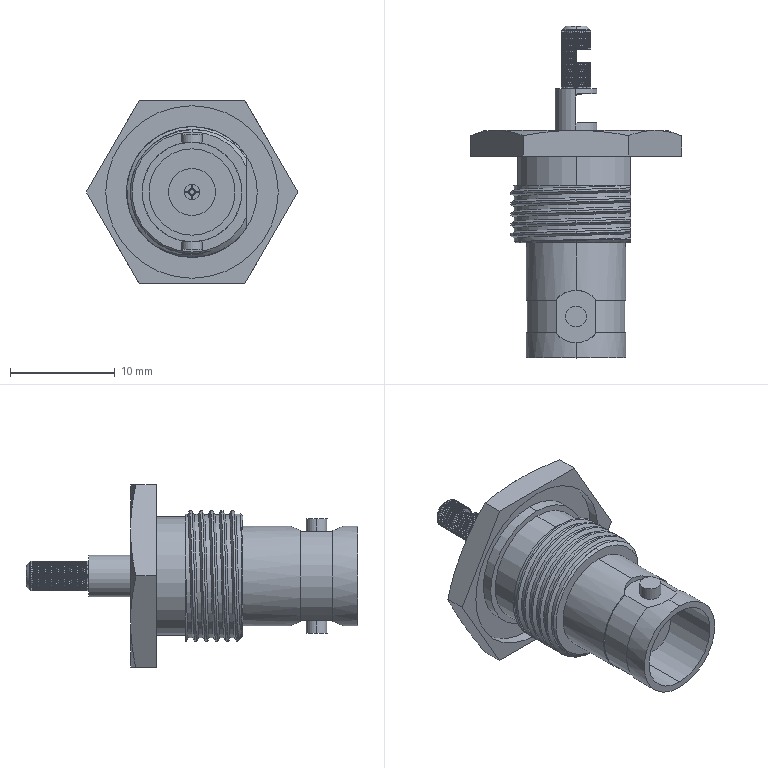Part | SolidWorks | features ICE 8, Helix 2, MirrorPattern 2, Revolution 2, SweepCut 2, CirPattern 1, Extrusion 1, RevCut 1 | 3 solids | 2054 faces | box 20.207 x 31.75 x 17.5 mm | volume 1414 mm3 | spline 1539 | cylinder 363 | plane 136 | cone 16 | commonest cylinder face diameters 2.8 x306 12.5 x18 2 x5 5 x4 9.55 x4 1.8 x3